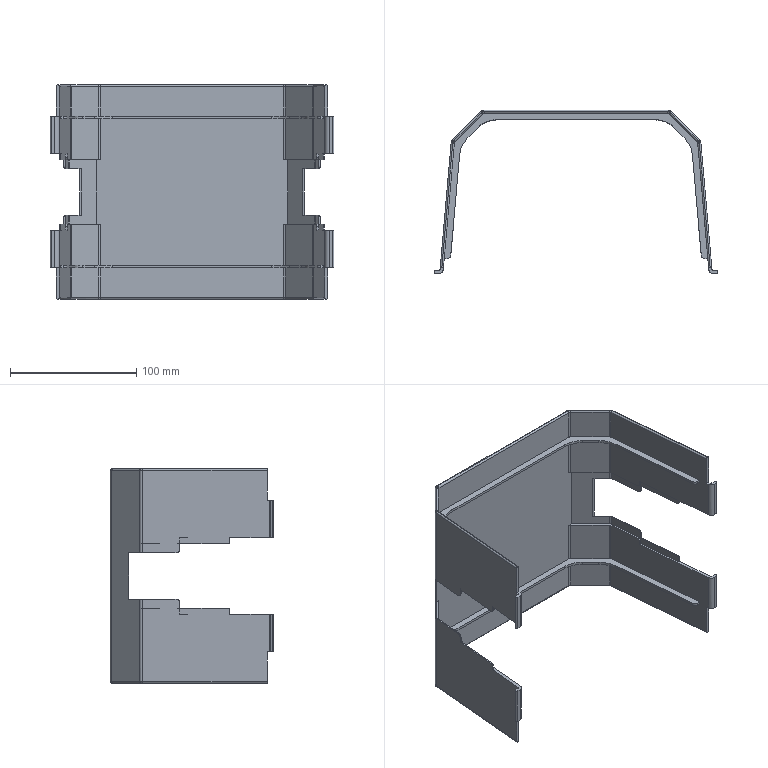Part | STEP file | 101000007620 | 1 solid | 202 faces | box 225 x 129.5 x 170 mm | volume 152398 mm3 | plane 100 | cylinder 86 | torus 16 | commonest cylinder face diameters 2.5 x28 4 x22 7 x10 6 x8 40 x8 2 x6